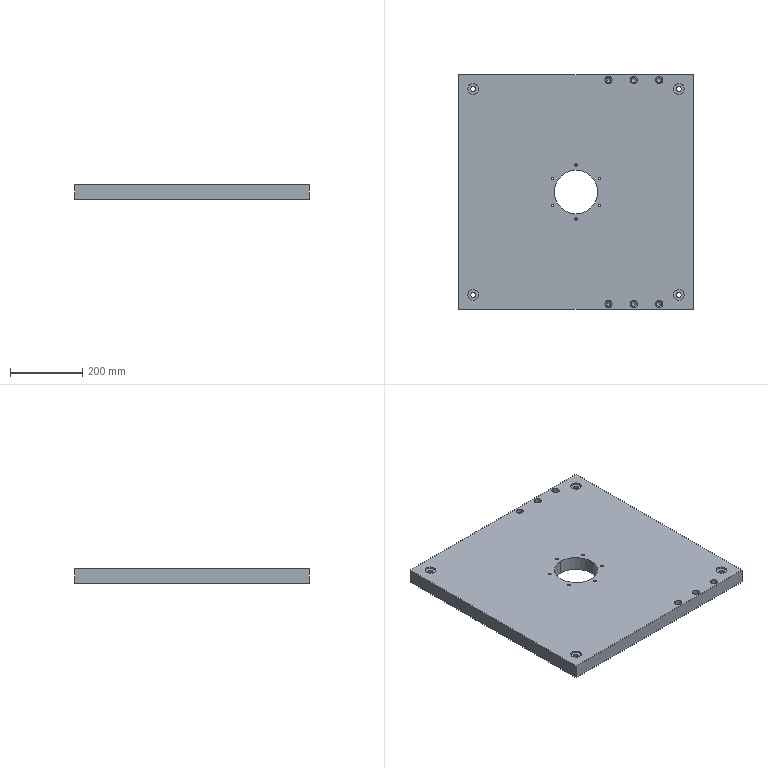Part | SolidWorks | features BaseBody 1 | 1 solid | 94 faces | box 650 x 650 x 40 mm | volume 16353197 mm3 | cylinder 62 | plane 20 | cone 12 | commonest cylinder face diameters 13.5 x20 20 x20 6.8 x12 30 x8 120 x2